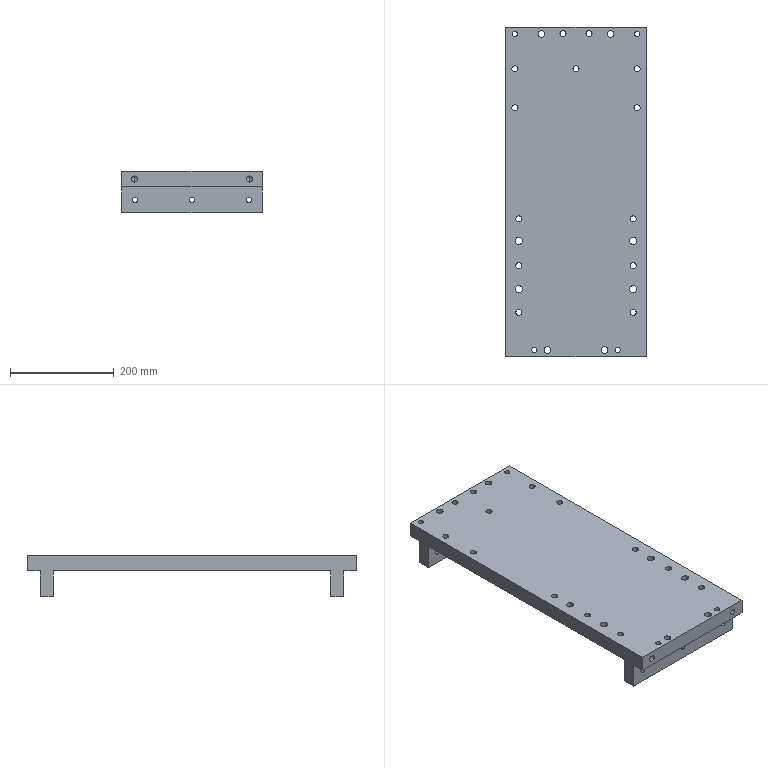Part | STEP file | MAT BAN GIUA | 1 solid | 92 faces | box 270 x 633.6 x 80 mm | volume 5694476 mm3 | cylinder 70 | plane 14 | cone 8 | commonest cylinder face diameters 11.835 x34 10.106 x20 13 x8 14 x8